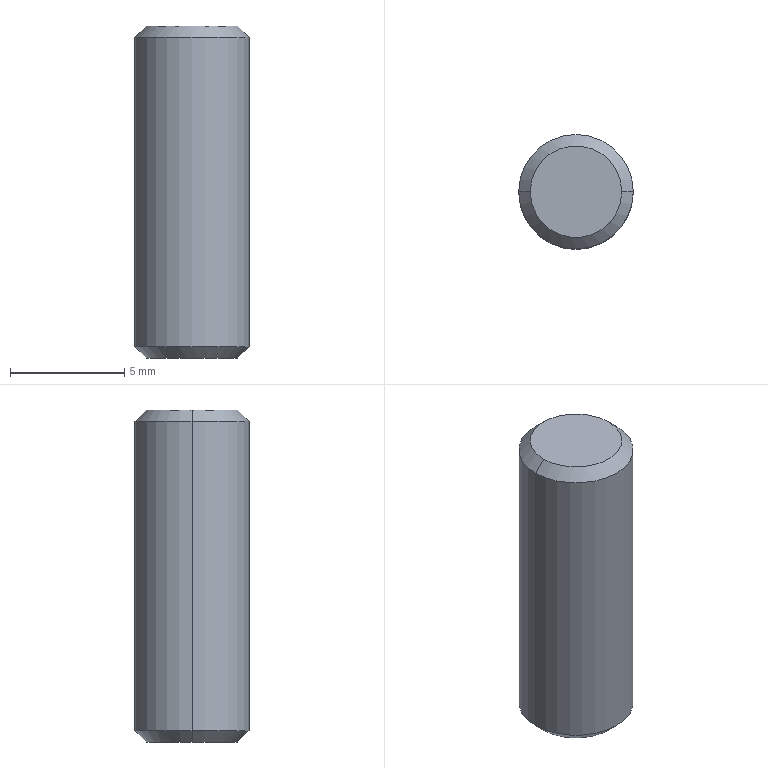Part | STEP file | FBDS-CS-010 | 1 solid | 8 faces | box 5 x 5 x 14.5 mm | volume 281.042 mm3 | cone 4 | cylinder 2 | plane 2 | commonest cylinder face diameters 5 x2
STEP:
#1=CARTESIAN_POINT('',(2.,0.,14.5));
#2=VERTEX_POINT('',#1);
#3=CARTESIAN_POINT('',(-2.,0.,14.5));
#4=VERTEX_POINT('',#3);
#5=CARTESIAN_POINT('',(0.,0.,14.5));
#6=DIRECTION('',(0.,0.,1.));
#7=DIRECTION('',(1.,0.,0.));
#8=AXIS2_PLACEMENT_3D('',#5,#6,#7);
#9=CIRCLE('',#8,2.);
#10=EDGE_CURVE('',#2,#4,#9,.T.);
#11=ORIENTED_EDGE('',*,*,#10,.F.);
#12=CARTESIAN_POINT('',(2.5,0.,14.));
#13=VERTEX_POINT('',#12);
#14=CARTESIAN_POINT('',(2.,0.,14.5));
#15=DIRECTION('',(0.7071,0.,-0.7071));
#16=VECTOR('',#15,1000.);
#17=LINE('',#14,#16);
#18=EDGE_CURVE('',#2,#13,#17,.T.);
#19=ORIENTED_EDGE('',*,*,#18,.T.);
#20=CARTESIAN_POINT('',(-2.5,0.,14.));
#21=VERTEX_POINT('',#20);
#22=CARTESIAN_POINT('',(0.,0.,14.));
#23=DIRECTION('',(0.,0.,-1.));
#24=DIRECTION('',(1.,0.,0.));
#25=AXIS2_PLACEMENT_3D('',#22,#23,#24);
#26=CIRCLE('',#25,2.5);
#27=EDGE_CURVE('',#21,#13,#26,.T.);
#28=ORIENTED_EDGE('',*,*,#27,.F.);
#29=CARTESIAN_POINT('',(-2.,0.,14.5));
#30=DIRECTION('',(-0.7071,0.,-0.7071));
#31=VECTOR('',#30,1000.);
#32=LINE('',#29,#31);
#33=EDGE_CURVE('',#4,#21,#32,.T.);
#34=ORIENTED_EDGE('',*,*,#33,.F.);
#35=EDGE_LOOP('',(#11,#19,#28,#34));
#36=FACE_OUTER_BOUND('',#35,.T.);
#37=CARTESIAN_POINT('',(0.,0.,14.5));
#38=DIRECTION('',(0.,0.,-1.));
#39=DIRECTION('',(-1.,0.,0.));
#40=AXIS2_PLACEMENT_3D('',#37,#38,#39);
#41=CONICAL_SURFACE('',#40,2.,0.7854);
#42=ADVANCED_FACE('',(#36),#41,.T.);
#43=CARTESIAN_POINT('',(-2.,0.,0.));
#44=VERTEX_POINT('',#43);
#45=CARTESIAN_POINT('',(2.,0.,0.));
#46=VERTEX_POINT('',#45);
#47=CARTESIAN_POINT('',(0.,0.,0.));
#48=DIRECTION('',(0.,0.,-1.));
#49=DIRECTION('',(1.,0.,0.));
#50=AXIS2_PLACEMENT_3D('',#47,#48,#49);
#51=CIRCLE('',#50,2.);
#52=EDGE_CURVE('',#44,#46,#51,.T.);
#53=ORIENTED_EDGE('',*,*,#52,.F.);
#54=CARTESIAN_POINT('',(-2.5,0.,0.5));
#55=VERTEX_POINT('',#54);
#56=CARTESIAN_POINT('',(-2.5,0.,0.5));
#57=DIRECTION('',(-0.7071,0.,0.7071));
#58=VECTOR('',#57,1000.);
#59=LINE('',#56,#58);
#60=EDGE_CURVE('',#44,#55,#59,.T.);
#61=ORIENTED_EDGE('',*,*,#60,.T.);
#62=CARTESIAN_POINT('',(2.5,0.,0.5));
#63=VERTEX_POINT('',#62);
#64=CARTESIAN_POINT('',(0.,0.,0.5));
#65=DIRECTION('',(0.,0.,1.));
#66=DIRECTION('',(1.,0.,0.));
#67=AXIS2_PLACEMENT_3D('',#64,#65,#66);
#68=CIRCLE('',#67,2.5);
#69=EDGE_CURVE('',#63,#55,#68,.T.);
#70=ORIENTED_EDGE('',*,*,#69,.F.);
#71=CARTESIAN_POINT('',(2.5,0.,0.5));
#72=DIRECTION('',(0.7071,0.,0.7071));
#73=VECTOR('',#72,1000.);
#74=LINE('',#71,#73);
#75=EDGE_CURVE('',#46,#63,#74,.T.);
#76=ORIENTED_EDGE('',*,*,#75,.F.);
#77=EDGE_LOOP('',(#53,#61,#70,#76));
#78=FACE_OUTER_BOUND('',#77,.T.);
#79=CARTESIAN_POINT('',(0.,0.,0.5));
#80=DIRECTION('',(0.,0.,1.));
#81=DIRECTION('',(1.,0.,0.));
#82=AXIS2_PLACEMENT_3D('',#79,#80,#81);
#83=CONICAL_SURFACE('',#82,2.5,0.7854);
#84=ADVANCED_FACE('',(#78),#83,.T.);
#85=ORIENTED_EDGE('',*,*,#27,.T.);
#86=CARTESIAN_POINT('',(2.5,0.,14.5));
#87=DIRECTION('',(0.,0.,-1.));
#88=VECTOR('',#87,1000.);
#89=LINE('',#86,#88);
#90=EDGE_CURVE('',#13,#63,#89,.T.);
#91=ORIENTED_EDGE('',*,*,#90,.T.);
#92=ORIENTED_EDGE('',*,*,#69,.T.);
#93=CARTESIAN_POINT('',(-2.5,0.,14.5));
#94=DIRECTION('',(0.,0.,-1.));
#95=VECTOR('',#94,1000.);
#96=LINE('',#93,#95);
#97=EDGE_CURVE('',#21,#55,#96,.T.);
#98=ORIENTED_EDGE('',*,*,#97,.F.);
#99=EDGE_LOOP('',(#85,#91,#92,#98));
#100=FACE_OUTER_BOUND('',#99,.T.);
#101=CARTESIAN_POINT('',(0.,0.,14.5));
#102=DIRECTION('',(0.,0.,-1.));
#103=DIRECTION('',(-1.,0.,0.));
#104=AXIS2_PLACEMENT_3D('',#101,#102,#103);
#105=CYLINDRICAL_SURFACE('',#104,2.5);
#106=ADVANCED_FACE('',(#100),#105,.T.);
#107=ORIENTED_EDGE('',*,*,#90,.F.);
#108=CARTESIAN_POINT('',(0.,0.,14.));
#109=DIRECTION('',(0.,0.,-1.));
#110=DIRECTION('',(1.,0.,0.));
#111=AXIS2_PLACEMENT_3D('',#108,#109,#110);
#112=CIRCLE('',#111,2.5);
#113=EDGE_CURVE('',#13,#21,#112,.T.);
#114=ORIENTED_EDGE('',*,*,#113,.T.);
#115=ORIENTED_EDGE('',*,*,#97,.T.);
#116=CARTESIAN_POINT('',(0.,0.,0.5));
#117=DIRECTION('',(0.,0.,1.));
#118=DIRECTION('',(1.,0.,0.));
#119=AXIS2_PLACEMENT_3D('',#116,#117,#118);
#120=CIRCLE('',#119,2.5);
#121=EDGE_CURVE('',#55,#63,#120,.T.);
#122=ORIENTED_EDGE('',*,*,#121,.T.);
#123=EDGE_LOOP('',(#107,#114,#115,#122));
#124=FACE_OUTER_BOUND('',#123,.T.);
#125=CARTESIAN_POINT('',(0.,0.,14.5));
#126=DIRECTION('',(0.,0.,-1.));
#127=DIRECTION('',(-1.,0.,0.));
#128=AXIS2_PLACEMENT_3D('',#125,#126,#127);
#129=CYLINDRICAL_SURFACE('',#128,2.5);
#130=ADVANCED_FACE('',(#124),#129,.T.);
#131=CARTESIAN_POINT('',(0.,0.,14.5));
#132=DIRECTION('',(0.,0.,1.));
#133=DIRECTION('',(1.,0.,0.));
#134=AXIS2_PLACEMENT_3D('',#131,#132,#133);
#135=CIRCLE('',#134,2.);
#136=EDGE_CURVE('',#4,#2,#135,.T.);
#137=ORIENTED_EDGE('',*,*,#136,.T.);
#138=ORIENTED_EDGE('',*,*,#10,.T.);
#139=EDGE_LOOP('',(#137,#138));
#140=FACE_OUTER_BOUND('',#139,.T.);
#141=CARTESIAN_POINT('',(0.,0.,14.5));
#142=DIRECTION('',(0.,0.,1.));
#143=DIRECTION('',(1.,0.,0.));
#144=AXIS2_PLACEMENT_3D('',#141,#142,#143);
#145=PLANE('',#144);
#146=ADVANCED_FACE('',(#140),#145,.T.);
#147=CARTESIAN_POINT('',(0.,0.,0.));
#148=DIRECTION('',(0.,0.,-1.));
#149=DIRECTION('',(1.,0.,0.));
#150=AXIS2_PLACEMENT_3D('',#147,#148,#149);
#151=CIRCLE('',#150,2.);
#152=EDGE_CURVE('',#46,#44,#151,.T.);
#153=ORIENTED_EDGE('',*,*,#152,.T.);
#154=ORIENTED_EDGE('',*,*,#52,.T.);
#155=EDGE_LOOP('',(#153,#154));
#156=FACE_OUTER_BOUND('',#155,.T.);
#157=CARTESIAN_POINT('',(0.,0.,0.));
#158=DIRECTION('',(0.,0.,1.));
#159=DIRECTION('',(1.,0.,0.));
#160=AXIS2_PLACEMENT_3D('',#157,#158,#159);
#161=PLANE('',#160);
#162=ADVANCED_FACE('',(#156),#161,.F.);
#163=ORIENTED_EDGE('',*,*,#60,.F.);
#164=ORIENTED_EDGE('',*,*,#152,.F.);
#165=ORIENTED_EDGE('',*,*,#75,.T.);
#166=ORIENTED_EDGE('',*,*,#121,.F.);
#167=EDGE_LOOP('',(#163,#164,#165,#166));
#168=FACE_OUTER_BOUND('',#167,.T.);
#169=CARTESIAN_POINT('',(0.,0.,0.5));
#170=DIRECTION('',(0.,0.,1.));
#171=DIRECTION('',(1.,0.,0.));
#172=AXIS2_PLACEMENT_3D('',#169,#170,#171);
#173=CONICAL_SURFACE('',#172,2.5,0.7854);
#174=ADVANCED_FACE('',(#168),#173,.T.);
#175=ORIENTED_EDGE('',*,*,#18,.F.);
#176=ORIENTED_EDGE('',*,*,#136,.F.);
#177=ORIENTED_EDGE('',*,*,#33,.T.);
#178=ORIENTED_EDGE('',*,*,#113,.F.);
#179=EDGE_LOOP('',(#175,#176,#177,#178));
#180=FACE_OUTER_BOUND('',#179,.T.);
#181=CARTESIAN_POINT('',(0.,0.,14.5));
#182=DIRECTION('',(0.,0.,-1.));
#183=DIRECTION('',(-1.,0.,0.));
#184=AXIS2_PLACEMENT_3D('',#181,#182,#183);
#185=CONICAL_SURFACE('',#184,2.,0.7854);
#186=ADVANCED_FACE('',(#180),#185,.T.);
#187=CLOSED_SHELL('',(#42,#84,#106,#130,#146,#162,#174,#186));
#188=MANIFOLD_SOLID_BREP('',#187);
#189=CARTESIAN_POINT('',(0.,0.,0.));
#190=DIRECTION('',(0.,0.,1.));
#191=DIRECTION('',(1.,0.,0.));
#192=AXIS2_PLACEMENT_3D('',#189,#190,#191);
#193=(LENGTH_UNIT()NAMED_UNIT(*)SI_UNIT(.MILLI.,.METRE.));
#194=UNCERTAINTY_MEASURE_WITH_UNIT(LENGTH_MEASURE(0.00001),#193,'','');
#195=(NAMED_UNIT(*)PLANE_ANGLE_UNIT()SI_UNIT($,.RADIAN.));
#196=(NAMED_UNIT(*)SI_UNIT($,.STERADIAN.)SOLID_ANGLE_UNIT());
#197=(GEOMETRIC_REPRESENTATION_CONTEXT(3)GLOBAL_UNCERTAINTY_ASSIGNED_CONTEXT((#194))GLOBAL_UNIT_ASSIGNED_CONTEXT((#193,#195,#196))REPRESENTATION_CONTEXT('',''));
#198=ADVANCED_BREP_SHAPE_REPRESENTATION('',(#188,#192),#197);